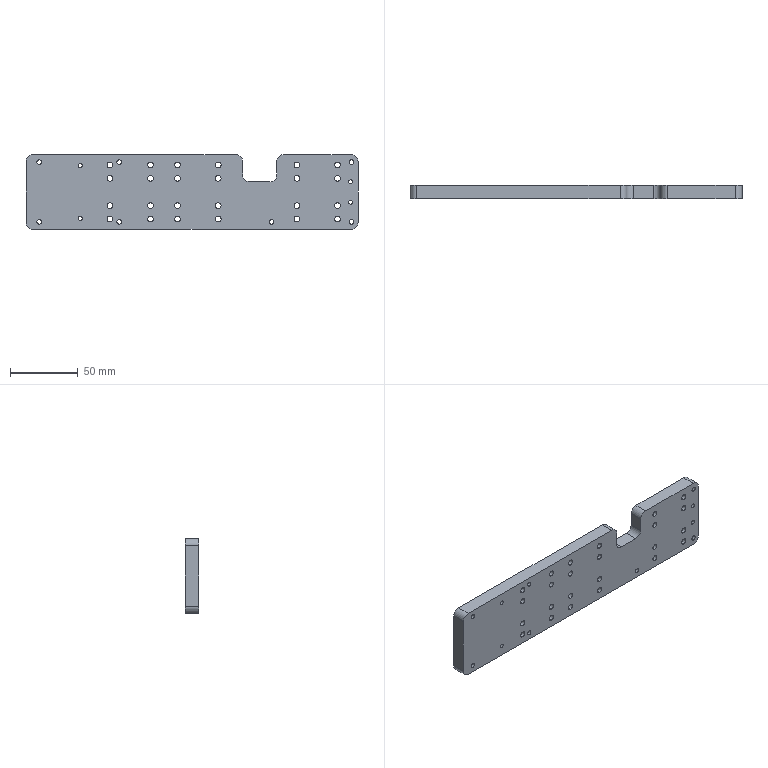Part | SolidWorks | features HoleWzd 2, Cut 1, Extrusion 1, LPattern 1 | 1 solid | 109 faces | box 245 x 10 x 55 mm | volume 124835 mm3 | cylinder 92 | plane 17 | commonest cylinder face diameters 4.2 x48 3.4 x14 6 x14 3 x8 10 x8